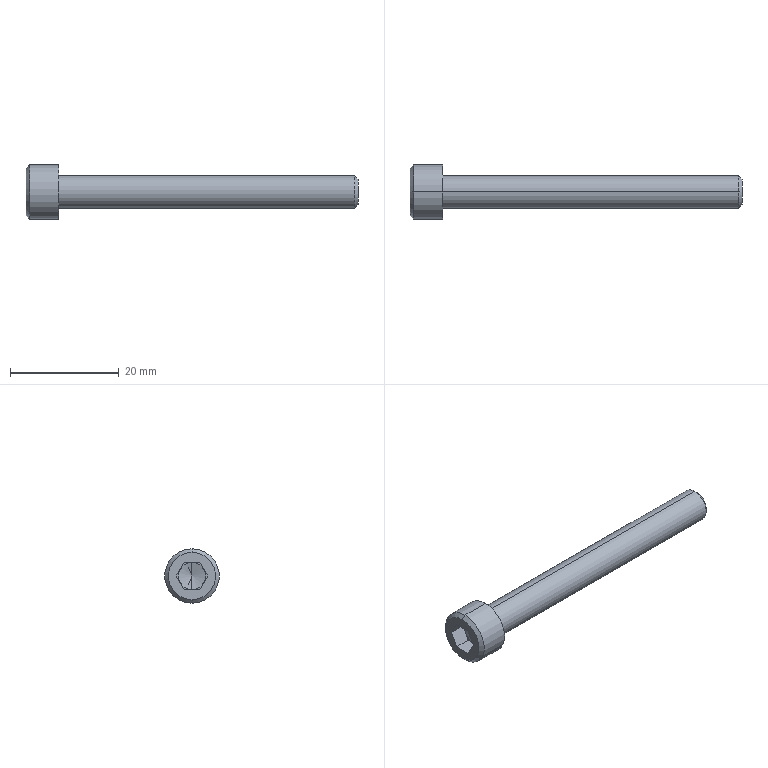Part | STEP file | 0230_305_SCB6-55 | 1 solid | 25 faces | box 61 x 10 x 10 mm | volume 1947 mm3 | plane 15 | cone 6 | cylinder 4 | commonest cylinder face diameters 6 x2 10 x2